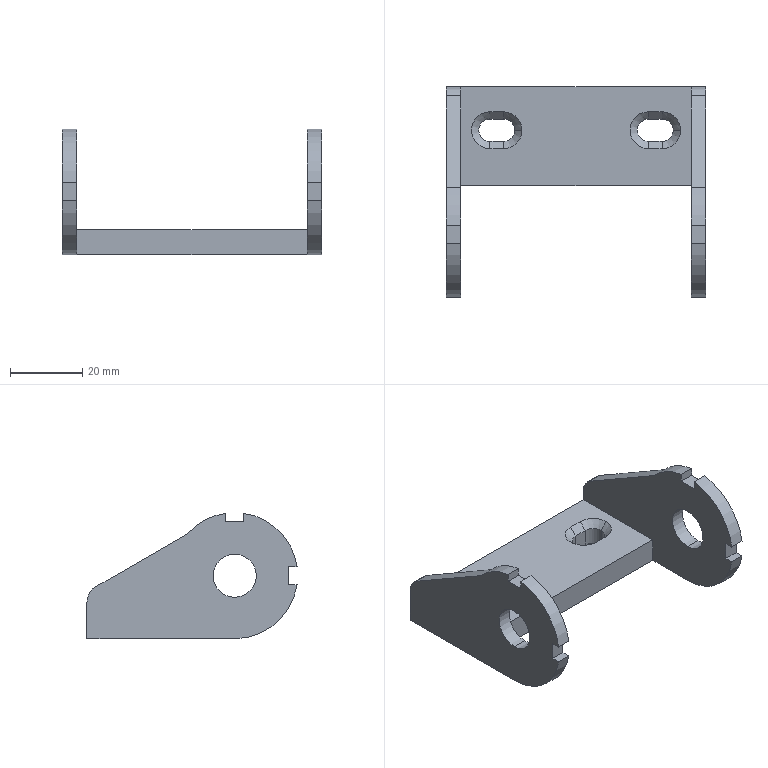Part | STEP file | TFH-FREE-END57 | 1 solid | 60 faces | box 72 x 58.321 x 34.821 mm | volume 22010 mm3 | plane 36 | cylinder 18 | cone 6 | commonest cylinder face diameters 6.2 x6 35 x6 12 x4 10 x2